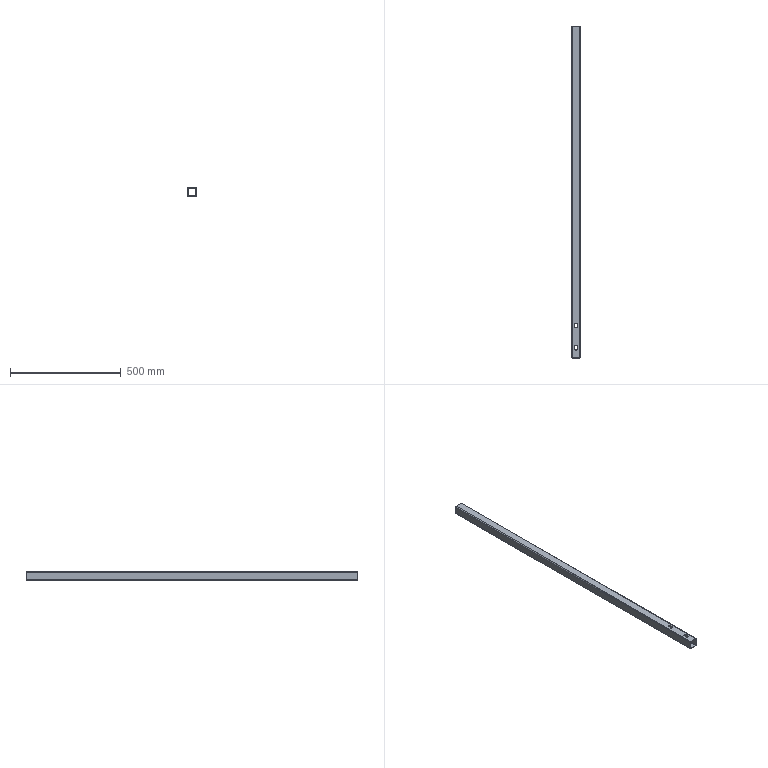Part | STEP file | 护栏立柱1主体_Default<As Machined> | 1 solid | 34 faces | box 40 x 1500 x 40 mm | volume 438684 mm3 | plane 18 | cylinder 16 | commonest cylinder face diameters 12 x8 4 x4 8 x4